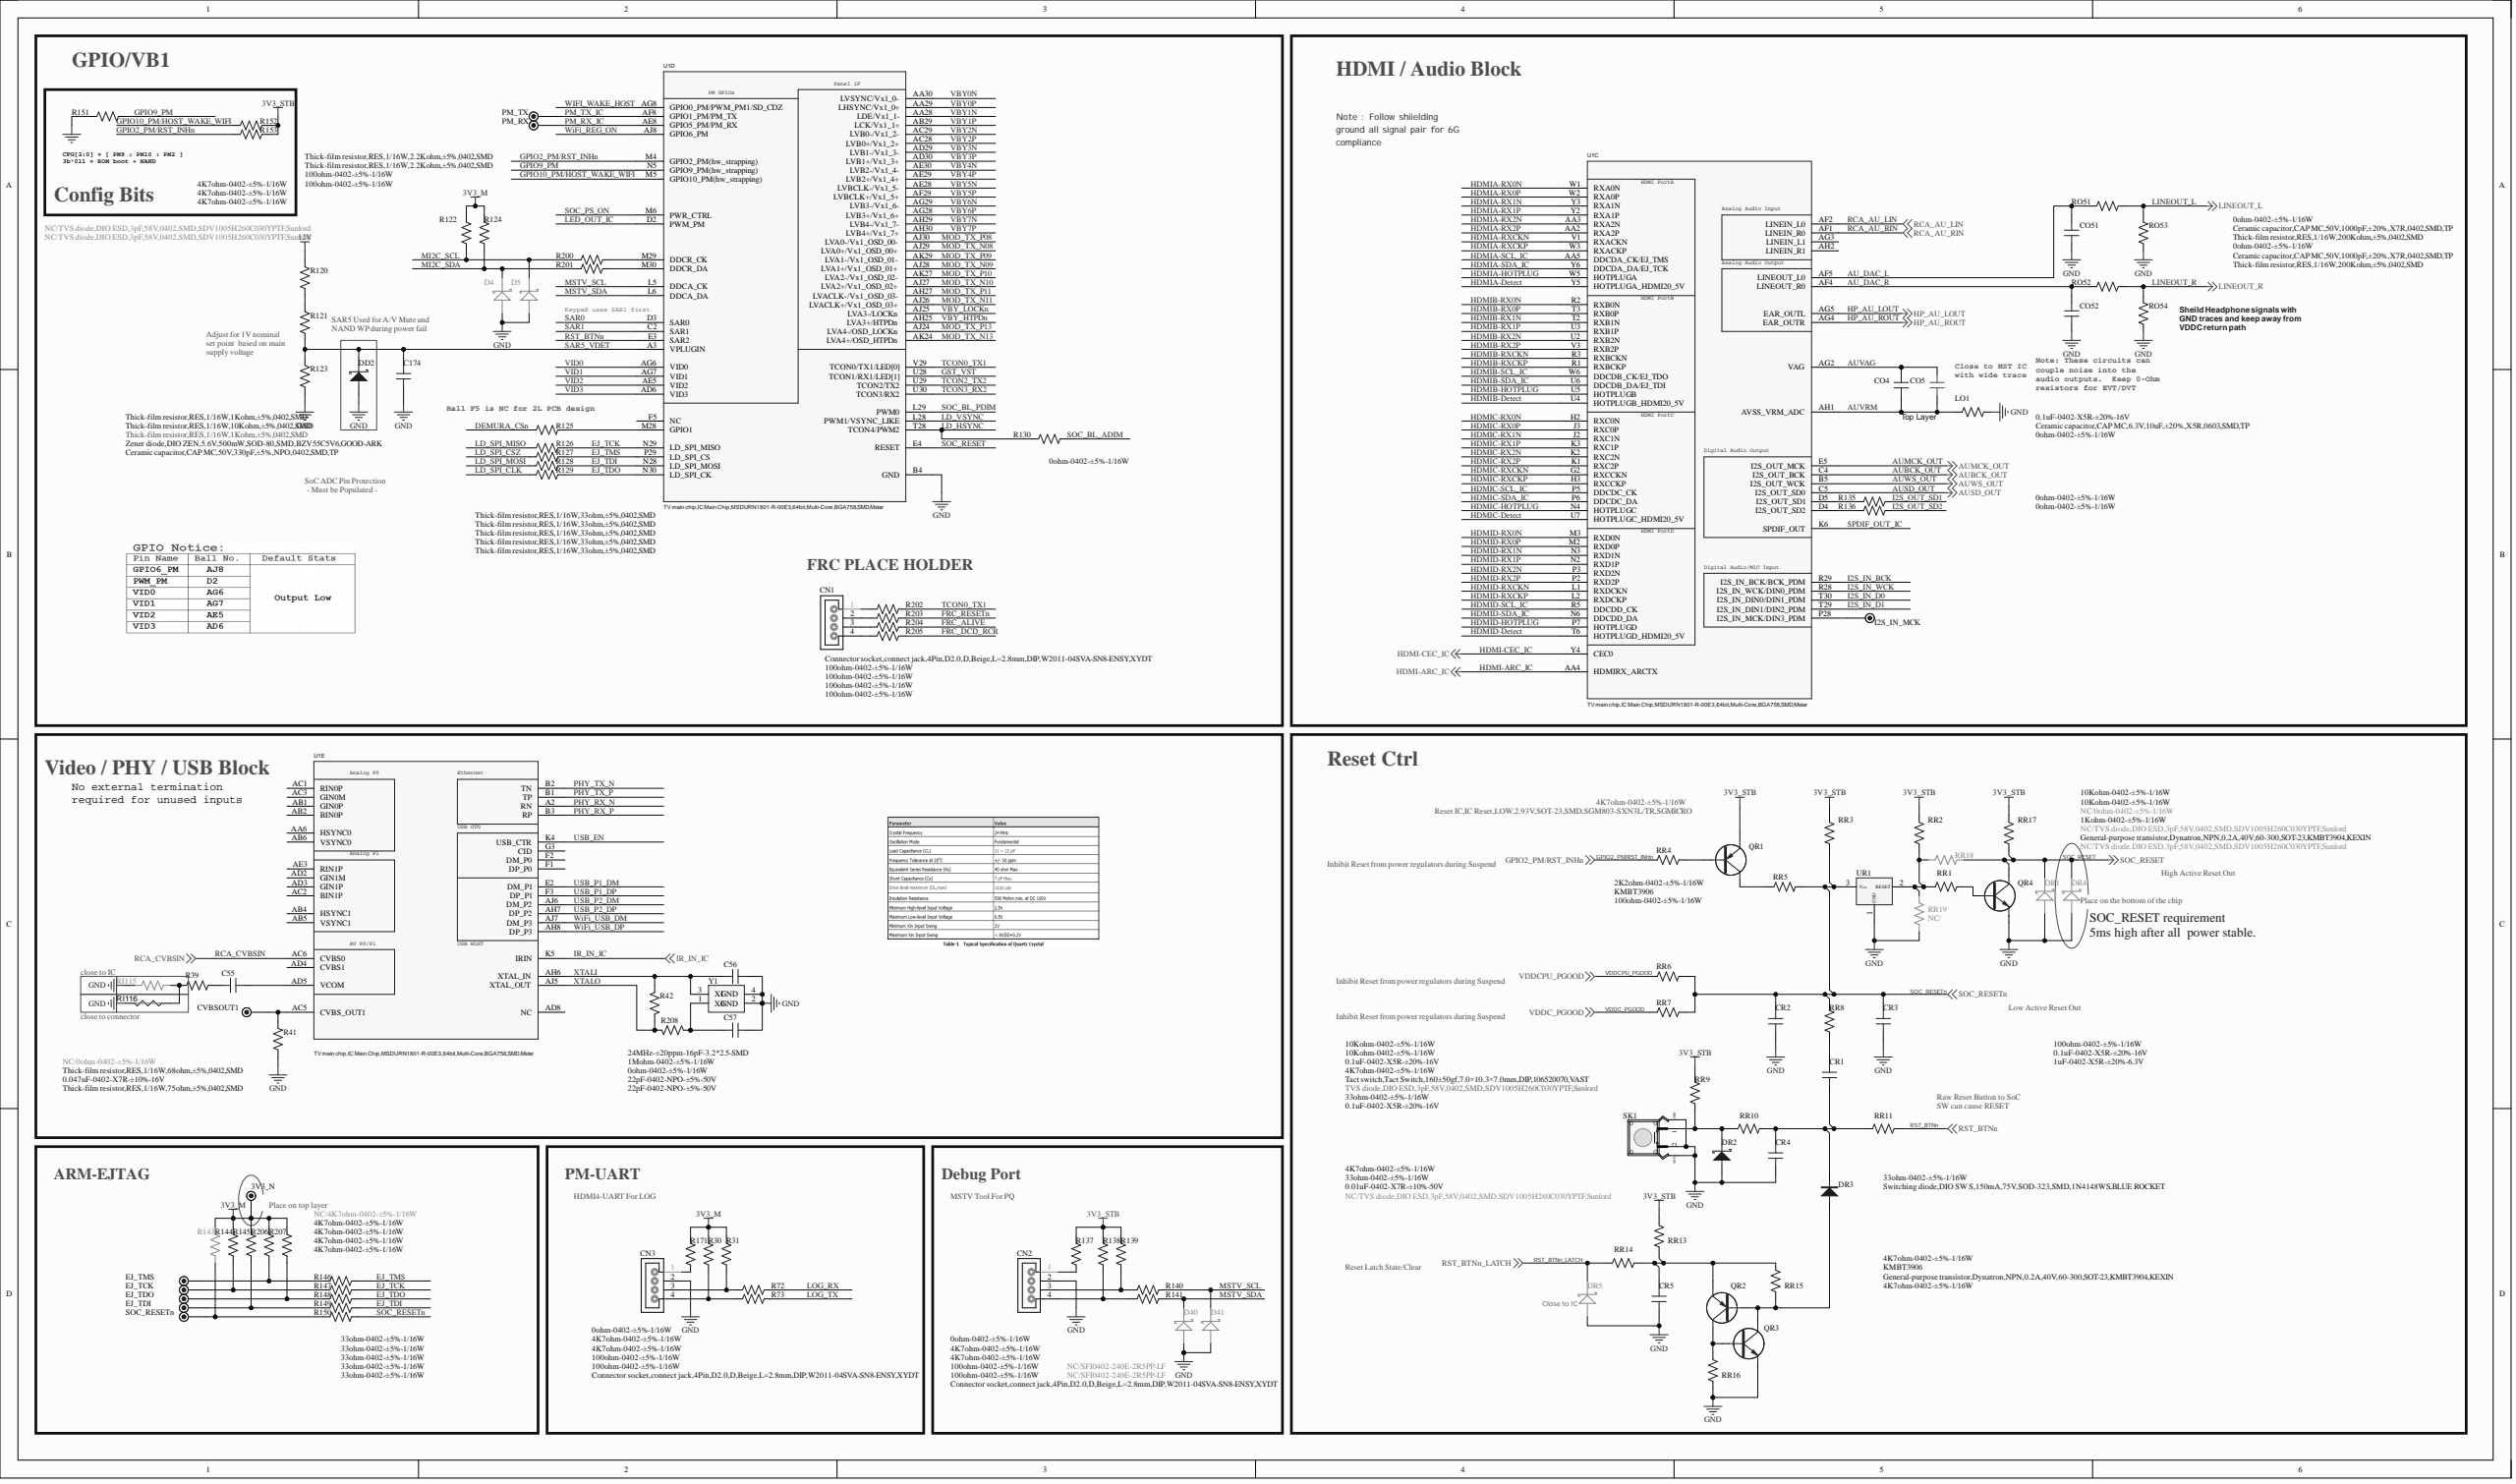Circuit board | Altium Designer | 1029 parts | 642 nets | one sheet of the schematic
Parts on this sheet (reference | value | footprint):
3V3_N | TEST | TP-20
C55 | 0.047uF-0402-X7R-±10%-16V | C0402
C56 | 22pF-0402-NPO-±5%-50V | C0402
C57 | 22pF-0402-NPO-±5%-50V | C0402
C174 | Ceramic capacitor,CAP MC,50V,330pF,±5%,NPO,0402,SMD,TP | C0402
CN1 | Connector socket,connect jack,4Pin,D2.0,D,Beige,L=2.8mm,DIP,W2011-04SVA-SN8-ENSY,XYDT | SIP4/2.0D-1
CN2 | Connector socket,connect jack,4Pin,D2.0,D,Beige,L=2.8mm,DIP,W2011-04SVA-SN8-ENSY,XYDT | SIP4/2.0D-1
CN3 | Connector socket,connect jack,4Pin,D2.0,D,Beige,L=2.8mm,DIP,W2011-04SVA-SN8-ENSY,XYDT | SIP4/2.0D-1
CO4 | 0.1uF-0402-X5R-±20%-16V | C0402
CO5 | Ceramic capacitor,CAP MC,6.3V,10uF,±20%,X5R,0603,SMD,TP | C0603
CO51 | Ceramic capacitor,CAP MC,50V,1000pF,±20%,X7R,0402,SMD,TP | C0402
CO52 | Ceramic capacitor,CAP MC,50V,1000pF,±20%,X7R,0402,SMD,TP | C0402
CR1 | 1uF-0402-X5R-±20%-6.3V | C0402
CR2 | 0.1uF-0402-X5R-±20%-16V | C0402
CR3 | 0.1uF-0402-X5R-±20%-16V | C0402
CR4 | 0.1uF-0402-X5R-±20%-16V | C0402
CR5 | 0.01uF-0402-X7R-±10%-50V | C0402
CVBSOUT1 | TEST | TP-20
D4 | NC/TVS diode,DIO ESD,3pF,58V,0402,SMD,SDV1005H260C030YPTF,Sunlord | DIODE-S0402
D5 | NC/TVS diode,DIO ESD,3pF,58V,0402,SMD,SDV1005H260C030YPTF,Sunlord | DIODE-S0402
D40 | NC/SFI0402-240E-2R5PP-LF | DIODE-S0402
D41 | NC/SFI0402-240E-2R5PP-LF | DIODE-S0402
DD2 | Zener diode,DIO ZEN,5.6V,500mW,SOD-80,SMD,BZV55C5V6,GOOD-ARK | DIODE-S0805
DR1 | NC/TVS diode,DIO ESD,3pF,58V,0402,SMD,SDV1005H260C030YPTF,Sunlord | DIODE-S0402
DR2 | TVS diode,DIO ESD,3pF,58V,0402,SMD,SDV1005H260C030YPTF,Sunlord | DIODE-S0402
DR3 | Switching diode,DIO SW S,150mA,75V,SOD-323,SMD,1N4148WS,BLUE ROCKET | DIODE-S-12
DR4 | NC/TVS diode,DIO ESD,3pF,58V,0402,SMD,SDV1005H260C030YPTF,Sunlord | DIODE-S0402
DR5 | NC/TVS diode,DIO ESD,3pF,58V,0402,SMD,SDV1005H260C030YPTF,Sunlord | DIODE-S0402
EJ_TCK | TEST | TP-20
EJ_TDI | TEST | TP-20
EJ_TDO | TEST | TP-20
EJ_TMS | TEST | TP-20
I2S_IN_MCK | TEST | TP-20
LO1 | 0ohm-0402-±5%-1/16W | R0402
PM_RX | TEST | TP-20
PM_TX | TEST | TP-20
QR1 | KMBT3906 | SOT-23
QR2 | KMBT3906 | SOT-23
QR3 | General-purpose transistor,Dynatron,NPN,0.2A,40V,60-300,SOT-23,KMBT3904,KEXIN | SOT-23
QR4 | General-purpose transistor,Dynatron,NPN,0.2A,40V,60-300,SOT-23,KMBT3904,KEXIN | SOT-23
R30 | 4K7ohm-0402-±5%-1/16W | R0402
R31 | 4K7ohm-0402-±5%-1/16W | R0402
R39 | Thick-film resistor,RES,1/16W,68ohm,±5%,0402,SMD | R0402
R41 | Thick-film resistor,RES,1/16W,75ohm,±5%,0402,SMD | R0402
R42 | 1Mohm-0402-±5%-1/16W | R0402
R72 | 100ohm-0402-±5%-1/16W | R0402
R73 | 100ohm-0402-±5%-1/16W | R0402
R120 | Thick-film resistor,RES,1/16W,1Kohm,±5%,0402,SMD | R0402
R121 | Thick-film resistor,RES,1/16W,10Kohm,±5%,0402,SMD | R0402
R122 | Thick-film resistor,RES,1/16W,2.2Kohm,±5%,0402,SMD | R0402
R123 | Thick-film resistor,RES,1/16W,1Kohm,±5%,0402,SMD | R0402
R124 | Thick-film resistor,RES,1/16W,2.2Kohm,±5%,0402,SMD | R0402
R125 | Thick-film resistor,RES,1/16W,33ohm,±5%,0402,SMD | R0402
R126 | Thick-film resistor,RES,1/16W,33ohm,±5%,0402,SMD | R0402
R127 | Thick-film resistor,RES,1/16W,33ohm,±5%,0402,SMD | R0402
R128 | Thick-film resistor,RES,1/16W,33ohm,±5%,0402,SMD | R0402
R129 | Thick-film resistor,RES,1/16W,33ohm,±5%,0402,SMD | R0402
R130 | 0ohm-0402-±5%-1/16W | R0402
R135 | 0ohm-0402-±5%-1/16W | R0402
R136 | 0ohm-0402-±5%-1/16W | R0402
R137 | 0ohm-0402-±5%-1/16W | R0402
R138 | 4K7ohm-0402-±5%-1/16W | R0402
R139 | 4K7ohm-0402-±5%-1/16W | R0402
R140 | 100ohm-0402-±5%-1/16W | R0402
R141 | 100ohm-0402-±5%-1/16W | R0402
R143 | NC/4K7ohm-0402-±5%-1/16W | R0402
R144 | 4K7ohm-0402-±5%-1/16W | R0402
R145 | 4K7ohm-0402-±5%-1/16W | R0402
R146 | 33ohm-0402-±5%-1/16W | R0402
R147 | 33ohm-0402-±5%-1/16W | R0402
R148 | 33ohm-0402-±5%-1/16W | R0402
R149 | 33ohm-0402-±5%-1/16W | R0402
R150 | 33ohm-0402-±5%-1/16W | R0402
R151 | 4K7ohm-0402-±5%-1/16W | R0402
R152 | 4K7ohm-0402-±5%-1/16W | R0402
R153 | 4K7ohm-0402-±5%-1/16W | R0402
R171 | 0ohm-0402-±5%-1/16W | R0402
R200 | 100ohm-0402-±5%-1/16W | R0402
R201 | 100ohm-0402-±5%-1/16W | R0402
R202 | 100ohm-0402-±5%-1/16W | R0402
R203 | 100ohm-0402-±5%-1/16W | R0402
R204 | 100ohm-0402-±5%-1/16W | R0402
R205 | 100ohm-0402-±5%-1/16W | R0402
R206 | 4K7ohm-0402-±5%-1/16W | R0402
R207 | 4K7ohm-0402-±5%-1/16W | R0402
R208 | 0ohm-0402-±5%-1/16W | R0402
RI115 | NC/0ohm-0402-±5%-1/16W | R0402
RI116 | NC/SHORT | GND
RO51 | 0ohm-0402-±5%-1/16W | R0402
RO52 | 0ohm-0402-±5%-1/16W | R0402
RO53 | Thick-film resistor,RES,1/16W,200Kohm,±5%,0402,SMD | R0402
RO54 | Thick-film resistor,RES,1/16W,200Kohm,±5%,0402,SMD | R0402
RR1 | 1Kohm-0402-±5%-1/16W | R0402
RR2 | 10Kohm-0402-±5%-1/16W | R0402
RR3 | 4K7ohm-0402-±5%-1/16W | R0402
RR4 | 2K2ohm-0402-±5%-1/16W | R0402
RR5 | 100ohm-0402-±5%-1/16W | R0402
RR6 | 10Kohm-0402-±5%-1/16W | R0402
RR7 | 10Kohm-0402-±5%-1/16W | R0402
RR8 | 100ohm-0402-±5%-1/16W | R0402
RR9 | 4K7ohm-0402-±5%-1/16W | R0402
RR10 | 33ohm-0402-±5%-1/16W | R0402
RR11 | 33ohm-0402-±5%-1/16W | R0402
RR13 | 4K7ohm-0402-±5%-1/16W | R0402
RR14 | 33ohm-0402-±5%-1/16W | R0402
RR15 | 4K7ohm-0402-±5%-1/16W | R0402
RR16 | 4K7ohm-0402-±5%-1/16W | R0402
RR17 | 10Kohm-0402-±5%-1/16W | R0402
RR18 | NC/0ohm-0402-±5%-1/16W | R0402
RR19 | NC/ | R0402
SK1 | Tact switch,Tact Switch,160±50gf,7.0×10.3×7.0mm,DIP,106520070,VAST | KEY-HD-6
SOC_RESETn | TEST | TP-20
U1 | TV main chip,IC Main Chip,MSDURN1801-R-00E3,64bit,Multi-Core,BGA758,SMD,Mstar | BGA758/0.65
U2 | DDR chip,IC DDR3,DDR3,2133M,16bit,256MB,2Gb,FBGA96,SMD,K4B2G1646F-BCNB,Samsung | BGA96/0.8-1
U3 | DDR chip,IC DDR3,DDR3,2133M,16bit,256MB,2Gb,FBGA96,SMD,K4B2G1646F-BCNB,Samsung | BGA96/0.8-1
UR1 | Reset IC,IC Reset,LOW,2.93V,SOT-23,SMD,SGM803-SXN3L/TR,SGMICRO | SOT-23-3-1
Y1 | 24MHz-±20ppm-16pF-3.2*2.5-SMD | XTAL-S-3
Nets of these parts (net: part-pin ...):
XTALO: R42-2 R208-1 U1-AJ5
XTALI: C56-1 R42-1 Y1-3 U1-AH6
WIFI_WAKE_HOST: U1-AG8
WiFi_USB_DP: U1-AH8
WiFi_USB_DM: U1-AJ7
WiFi_REG_ON: U1-AJ8
VID3: U1-AD6
VID2: U1-AE5
VID1: U1-AG7
VID0: U1-AG6
VDDCPU_PGOOD: RR6-2
VDDC_PGOOD: RR7-2
VBY_LOCKn: U1-AJ25
VBY_HTPDn: U1-AH25
VBY7P: U1-AH30
VBY7N: U1-AH29
VBY6P: U1-AG28
VBY6N: U1-AG29
VBY5P: U1-AF29
VBY5N: U1-AE28
VBY4P: U1-AE29
VBY4N: U1-AE30
VBY3P: U1-AD30
VBY3N: U1-AD29
VBY2P: U1-AC28
VBY2N: U1-AC29
VBY1P: U1-AB29
VBY1N: U1-AA28
VBY0P: U1-AA29
VBY0N: U1-AA30
USB_P2_DP: U1-AH7
USB_P2_DM: U1-AJ6
USB_P1_DP: U1-F3
USB_P1_DM: U1-E2
USB_EN: U1-K4
TCON0_TX1: R202-2 U1-V29
SPDIF_OUT_IC: U1-K6
SOC_RESETn: CR2-2 CR3-2 R150-1 RR3-1 RR5-1 RR6-1 RR7-1 RR8-2 UR1-3
SOC_RESET: DR1-K DR4-K QR4-C RR17-1 RR18-2 U1-E4
SOC_PS_ON: U1-M6
SOC_BL_PDIM: U1-L29
SOC_BL_ADIM: R130-2
SAR5_VDET: C174-2 DD2-K R121-1 R123-2 U1-A3
SAR1: U1-C2
SAR0: U1-D3
RST_BTNn_LATCH: DR5-K RR14-2
RST_BTNn: RR11-1 U1-E3
RCA_CVBSIN: U1-AC6
RCA_AU_RIN: U1-AF1
RCA_AU_LIN: U1-AF2
PM_TX_IC: PM_TX-1 U1-AF8
PM_RX_IC: PM_RX-1 U1-AE8
PHY_TX_P: U1-B1
PHY_TX_N: U1-B2
PHY_RX_P: U1-B3
PHY_RX_N: U1-A2
NetRR1_2: RR1-2 RR2-1 RR18-1 RR19-1 UR1-2
NetR201_2: R201-2 U1-M30
NetR200_2: R200-2 U1-M29
NetR143_1: R143-1 R150-2 SOC_RESETn-1
NetR136_1: R136-1 U1-D4
NetR135_1: R135-1 U1-D5
NetR125_1: R125-1 U1-M28
NetR120_1: R120-1 R121-2
NetR39_1: R39-1 RI115-2 RI116-JP_2K
NetQR4_B: QR4-B RR1-1
NetQR2_C: QR2-C QR3-B RR16-2
NetQR1_C: QR1-C RR5-2
NetQR1_B: QR1-B RR4-2
NetI2S_IN_MCK_1: I2S_IN_MCK-1 U1-P28
NetEJ_TMS_1: EJ_TMS-1 R146-2 R206-1
NetEJ_TDO_1: EJ_TDO-1 R148-2 R207-1
NetEJ_TDI_1: EJ_TDI-1 R145-1 R149-2
NetEJ_TCK_1: EJ_TCK-1 R144-1 R147-2
NetDR3_A: DR3-A QR2-B QR3-C RR15-1
NetDR2_K: DR2-K RR9-1 RR10-2 SK1-2
NetCVBSOUT1_1: CVBSOUT1-1 R41-2 U1-AC5
NetCR5_2: CR5-2 QR2-E RR13-1 RR14-1 RR15-2
NetCR1_2: CR1-2 RR8-1
NetCR1_1: CR1-1 CR4-2 DR3-K RR10-1 RR11-2
NetCN3_4: CN3-4 R30-1 R73-1
NetCN3_3: CN3-3 R31-1 R72-1
NetCN3_1: CN3-1 R171-1
NetCN2_4: CN2-4 R138-1 R141-1
NetCN2_3: CN2-3 R139-1 R140-1
NetCN2_1: CN2-1 R137-1
NetCN1_4: CN1-4 R205-1
NetCN1_3: CN1-3 R204-1
NetCN1_2: CN1-2 R203-1
NetCN1_1: CN1-1 R202-1
NetC57_1: C57-1 R208-2 Y1-1
NetC55_2: C55-2 U1-AD5
NetC55_1: C55-1 R39-2
MSTV_SDA: D40-K R141-2 U1-L6
MSTV_SCL: D41-K R140-2 U1-L5
MI2C_SDA: D4-K R124-1 R201-1
MI2C_SCL: D5-K R122-1 R200-1
LOG_TX: R73-2
LOG_RX: R72-2
LINEOUT_R: RO52-2 RO54-2
LINEOUT_L: RO51-2 RO53-2
LED_OUT_IC: U1-D2
LD_VSYNC: U1-L28
LD_SPI_MOSI: R128-2
LD_SPI_MISO: R126-2
LD_SPI_CSZ: R127-2
LD_SPI_CLK: R129-2
LD_HSYNC: R130-1 U1-T28
IR_IN_IC: U1-K5
I2S_OUT_SD2: R136-2
I2S_OUT_SD1: R135-2
HP_AU_ROUT: U1-AG4
HP_AU_LOUT: U1-AG5
HDMID-SDA_IC: U1-N6
HDMID-SCL_IC: U1-R5
HDMID-RXCKP: U1-L2
HDMID-RXCKN: U1-L1
HDMID-RX2P: U1-P2
HDMID-RX2N: U1-P3
HDMID-RX1P: U1-N2
HDMID-RX1N: U1-N3
HDMID-RX0P: U1-M2
HDMID-RX0N: U1-M3
HDMID-HOTPLUG: U1-P7
HDMID-Detect: U1-T6
HDMIC-SDA_IC: U1-P6
HDMIC-SCL_IC: U1-P5
HDMIC-RXCKP: U1-H3
HDMIC-RXCKN: U1-G2
HDMIC-RX2P: U1-K1
HDMIC-RX2N: U1-K2
HDMIC-RX1P: U1-K3
HDMIC-RX1N: U1-J2
HDMIC-RX0P: U1-J3
HDMIC-RX0N: U1-H2
HDMIC-HOTPLUG: U1-N4
HDMIC-Detect: U1-U7
HDMIB-SDA_IC: U1-U6
HDMIB-SCL_IC: U1-W6
HDMIB-RXCKP: U1-R1
HDMIB-RXCKN: U1-R3
HDMIB-RX2P: U1-V3
HDMIB-RX2N: U1-U2
HDMIB-RX1P: U1-U3
HDMIB-RX1N: U1-T2
HDMIB-RX0P: U1-T3
HDMIB-RX0N: U1-R2
HDMIB-HOTPLUG: U1-U5
HDMIB-Detect: U1-U4
HDMIA-SDA_IC: U1-Y6
HDMIA-SCL_IC: U1-AA5
HDMIA-RXCKP: U1-W3
HDMIA-RXCKN: U1-V1
HDMIA-RX2P: U1-AA2
HDMIA-RX2N: U1-AA3
HDMIA-RX1P: U1-Y2
HDMIA-RX1N: U1-Y3
HDMIA-RX0P: U1-W2
HDMIA-RX0N: U1-W1
HDMIA-HOTPLUG: U1-W5
HDMIA-Detect: U1-Y5
HDMI-CEC_IC: U1-Y4
HDMI-ARC_IC: U1-AA4
GPIO10_PM/HOST_WAKE_WIFI: R152-2 U1-M5
GPIO9_PM: R151-1 U1-N5
GPIO2_PM/RST_INHn: R153-2 RR4-1 U1-M4
GND: C56-2 C57-2 C174-1 CN2-2 CN3-2 CO51-1 CO52-1 CR2-1 CR3-1 CR4-1 CR5-1 D4-A D5-A D40-A D41-A DD2-A DR1-A DR2-A DR4-A DR5-A LO1-2 QR3-E QR4-E R41-1 R123-1 R151-2 RI115-1 RI116-JP_1K RO53-1 RO54-1 RR16-1 RR19-2 SK1-1 SK1-3 SK1-4 UR1-1 Y1-2 Y1-4 U1-B4 U1-P1 U2-B1 U2-B3 U2-E2 U2-J2 U2-P1 U3-B1 U3-B3 U3-E2 U3-J2 U3-P1
FRC_RESETn: R203-2
FRC_DCD_RCR: R205-2
FRC_ALIVE: R204-2
EJ_TMS: R127-1 R146-1 U1-P29
EJ_TDO: R129-1 R148-1 U1-N30
EJ_TDI: R128-1 R149-1 U1-N28
EJ_TCK: R126-1 R147-1 U1-N29
DEMURA_CSn: R125-2
AUWS_OUT: U1-B5
AUVRM: CO4-1 CO5-1 LO1-1 U1-AH1
AUVAG: CO4-2 CO5-2 U1-AG2
AUSD_OUT: U1-C5
AUMCK_OUT: U1-E5
AUBCK_OUT: U1-C4
AU_DAC_R: CO52-2 RO52-1 U1-AF4
AU_DAC_L: CO51-2 RO51-1 U1-AF5
12V: R120-2
3V3_STB: QR1-E R137-2 R138-2 R139-2 R152-1 R153-1 RR2-2 RR3-2 RR9-2 RR13-2 RR17-2
3V3_M: 3V3_N-1 R30-2 R31-2 R122-2 R124-2 R143-2 R144-2 R145-2 R171-2 R206-2 R207-2